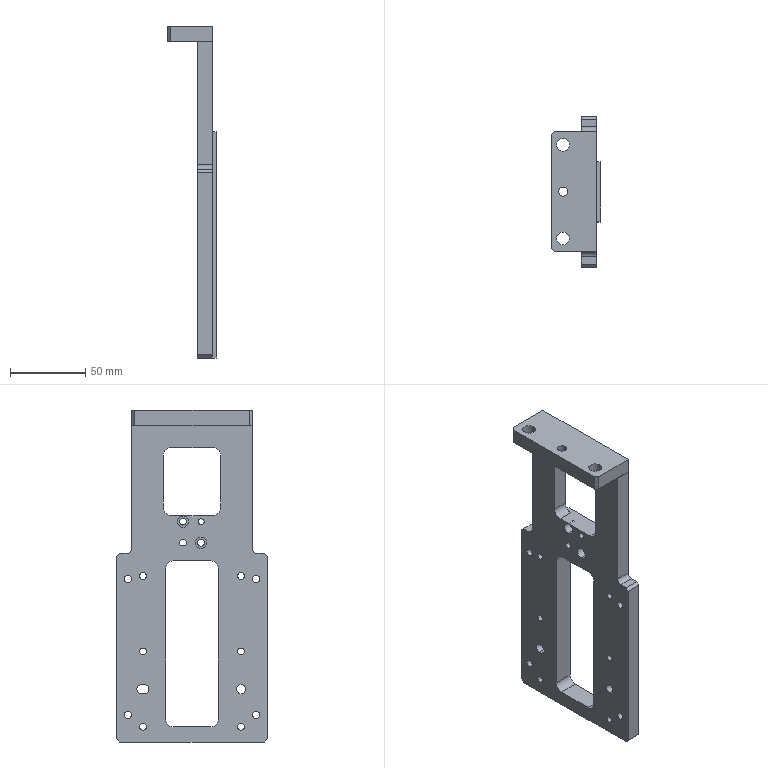Part | SolidWorks | features ICE 12, Chamfer 3, HoleWzd 3, Cut 2, Fillet 2, 3DProfileFeature 1, Extrusion 1 | 2 solids | 111 faces | box 33 x 100 x 220 mm | volume 162371 mm3 | cylinder 64 | plane 47 | commonest cylinder face diameters 4.5 x16 8 x12 5 x8 6 x8 10 x8 4 x4